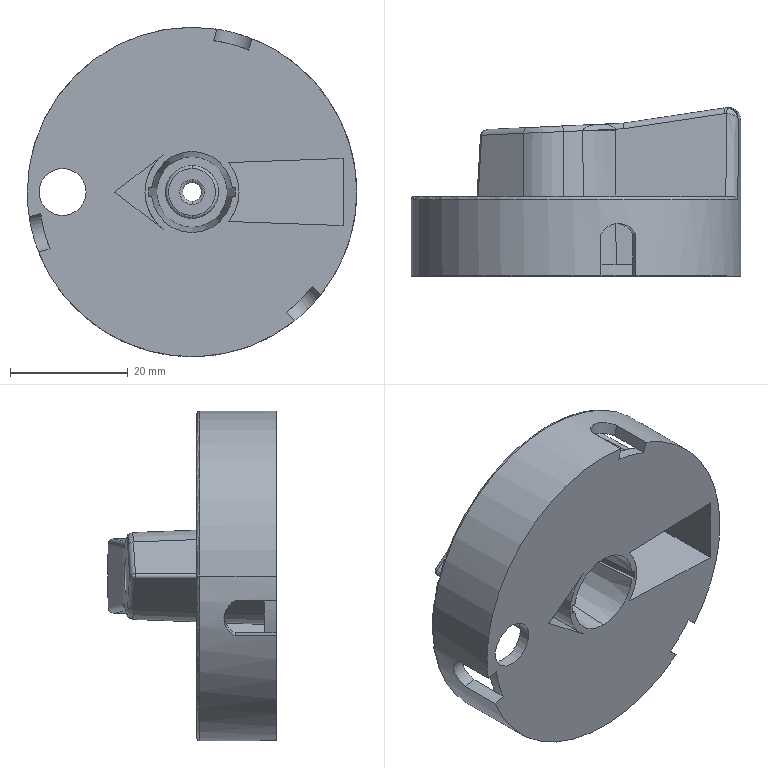Part | STEP file | PCS-P05A-001-2_1_2.stp | 1 solid | 103 faces | box 56 x 28.677 x 56 mm | volume 12848 mm3 | cylinder 37 | plane 37 | spline 18 | torus 8 | cone 3 | commonest cylinder face diameters 2 x9 16 x5 52 x4 6.958 x3 40 x3 3.2 x2